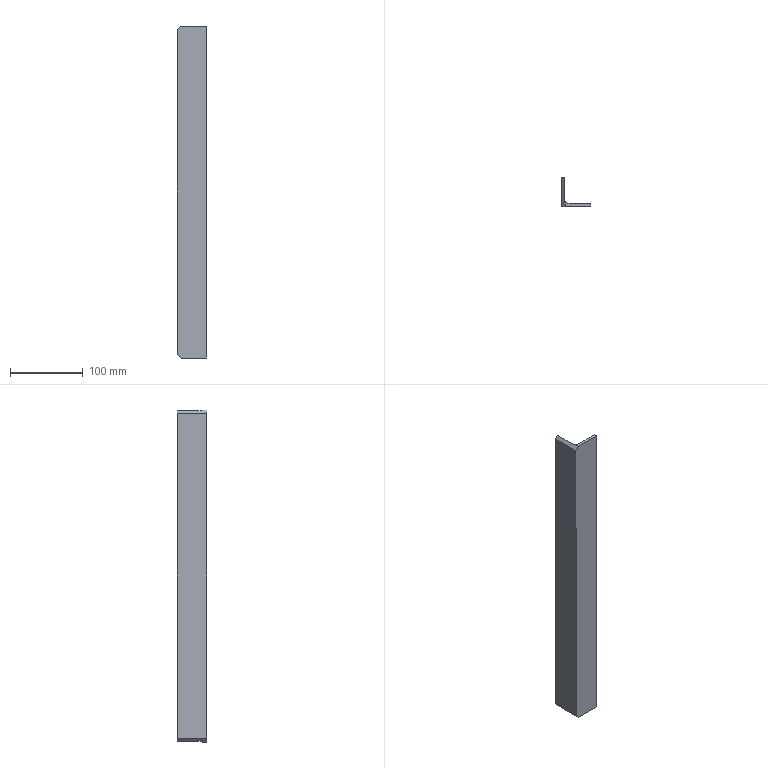Part | SolidWorks | features Cut 1, Extrusion 1 | 1 solid | 13 faces | box 40 x 40 x 456 mm | volume 140103 mm3 | plane 10 | cylinder 3 | commonest cylinder face diameters 0.02 x2 10 x1
STEP:
#1=CARTESIAN_POINT('',(0.,0.,451.));
#2=VERTEX_POINT('',#1);
#3=CARTESIAN_POINT('',(0.,0.,5.));
#4=VERTEX_POINT('',#3);
#5=CARTESIAN_POINT('',(0.,0.,456.));
#6=DIRECTION('',(0.,0.,-1.));
#7=VECTOR('',#6,1000.);
#8=LINE('',#5,#7);
#9=EDGE_CURVE('',#2,#4,#8,.T.);
#10=ORIENTED_EDGE('',*,*,#9,.T.);
#11=CARTESIAN_POINT('',(5.,0.,0.));
#12=VERTEX_POINT('',#11);
#13=CARTESIAN_POINT('',(0.,0.,5.));
#14=DIRECTION('',(0.7071,0.,-0.7071));
#15=VECTOR('',#14,1000.);
#16=LINE('',#13,#15);
#17=EDGE_CURVE('',#4,#12,#16,.T.);
#18=ORIENTED_EDGE('',*,*,#17,.T.);
#19=CARTESIAN_POINT('',(40.,0.,0.));
#20=VERTEX_POINT('',#19);
#21=CARTESIAN_POINT('',(40.,0.,0.));
#22=DIRECTION('',(1.,0.,0.));
#23=VECTOR('',#22,1000.);
#24=LINE('',#21,#23);
#25=EDGE_CURVE('',#12,#20,#24,.T.);
#26=ORIENTED_EDGE('',*,*,#25,.T.);
#27=CARTESIAN_POINT('',(40.,0.,456.));
#28=VERTEX_POINT('',#27);
#29=CARTESIAN_POINT('',(40.,0.,456.));
#30=DIRECTION('',(0.,0.,-1.));
#31=VECTOR('',#30,1000.);
#32=LINE('',#29,#31);
#33=EDGE_CURVE('',#28,#20,#32,.T.);
#34=ORIENTED_EDGE('',*,*,#33,.F.);
#35=CARTESIAN_POINT('',(5.,0.,456.));
#36=VERTEX_POINT('',#35);
#37=CARTESIAN_POINT('',(40.,0.,456.));
#38=DIRECTION('',(1.,0.,0.));
#39=VECTOR('',#38,1000.);
#40=LINE('',#37,#39);
#41=EDGE_CURVE('',#36,#28,#40,.T.);
#42=ORIENTED_EDGE('',*,*,#41,.F.);
#43=CARTESIAN_POINT('',(5.,0.,456.));
#44=DIRECTION('',(-0.7071,0.,-0.7071));
#45=VECTOR('',#44,1000.);
#46=LINE('',#43,#45);
#47=EDGE_CURVE('',#36,#2,#46,.T.);
#48=ORIENTED_EDGE('',*,*,#47,.T.);
#49=EDGE_LOOP('',(#10,#18,#26,#34,#42,#48));
#50=FACE_OUTER_BOUND('',#49,.T.);
#51=CARTESIAN_POINT('',(40.,0.,456.));
#52=DIRECTION('',(0.,1.,0.));
#53=DIRECTION('',(-1.,0.,0.));
#54=AXIS2_PLACEMENT_3D('',#51,#52,#53);
#55=PLANE('',#54);
#56=ADVANCED_FACE('',(#50),#55,.F.);
#57=CARTESIAN_POINT('',(40.,3.99,0.));
#58=VERTEX_POINT('',#57);
#59=CARTESIAN_POINT('',(40.,3.99,0.));
#60=DIRECTION('',(0.,1.,0.));
#61=VECTOR('',#60,1000.);
#62=LINE('',#59,#61);
#63=EDGE_CURVE('',#20,#58,#62,.T.);
#64=ORIENTED_EDGE('',*,*,#63,.T.);
#65=CARTESIAN_POINT('',(40.,3.99,456.));
#66=VERTEX_POINT('',#65);
#67=CARTESIAN_POINT('',(40.,3.99,456.));
#68=DIRECTION('',(0.,0.,-1.));
#69=VECTOR('',#68,1000.);
#70=LINE('',#67,#69);
#71=EDGE_CURVE('',#66,#58,#70,.T.);
#72=ORIENTED_EDGE('',*,*,#71,.F.);
#73=CARTESIAN_POINT('',(40.,3.99,456.));
#74=DIRECTION('',(0.,1.,0.));
#75=VECTOR('',#74,1000.);
#76=LINE('',#73,#75);
#77=EDGE_CURVE('',#28,#66,#76,.T.);
#78=ORIENTED_EDGE('',*,*,#77,.F.);
#79=ORIENTED_EDGE('',*,*,#33,.T.);
#80=EDGE_LOOP('',(#64,#72,#78,#79));
#81=FACE_OUTER_BOUND('',#80,.T.);
#82=CARTESIAN_POINT('',(40.,3.99,456.));
#83=DIRECTION('',(-1.,0.,0.));
#84=DIRECTION('',(0.,0.,1.));
#85=AXIS2_PLACEMENT_3D('',#82,#83,#84);
#86=PLANE('',#85);
#87=ADVANCED_FACE('',(#81),#86,.F.);
#88=CARTESIAN_POINT('',(39.99,4.,0.));
#89=VERTEX_POINT('',#88);
#90=CARTESIAN_POINT('',(39.99,3.99,0.));
#91=DIRECTION('',(0.,0.,1.));
#92=DIRECTION('',(1.,0.,0.));
#93=AXIS2_PLACEMENT_3D('',#90,#91,#92);
#94=CIRCLE('',#93,0.01);
#95=EDGE_CURVE('',#58,#89,#94,.T.);
#96=ORIENTED_EDGE('',*,*,#95,.T.);
#97=CARTESIAN_POINT('',(39.99,4.,456.));
#98=VERTEX_POINT('',#97);
#99=CARTESIAN_POINT('',(39.99,4.,456.));
#100=DIRECTION('',(0.,0.,-1.));
#101=VECTOR('',#100,1000.);
#102=LINE('',#99,#101);
#103=EDGE_CURVE('',#98,#89,#102,.T.);
#104=ORIENTED_EDGE('',*,*,#103,.F.);
#105=CARTESIAN_POINT('',(39.99,3.99,456.));
#106=DIRECTION('',(0.,0.,1.));
#107=DIRECTION('',(1.,0.,0.));
#108=AXIS2_PLACEMENT_3D('',#105,#106,#107);
#109=CIRCLE('',#108,0.01);
#110=EDGE_CURVE('',#66,#98,#109,.T.);
#111=ORIENTED_EDGE('',*,*,#110,.F.);
#112=ORIENTED_EDGE('',*,*,#71,.T.);
#113=EDGE_LOOP('',(#96,#104,#111,#112));
#114=FACE_OUTER_BOUND('',#113,.T.);
#115=CARTESIAN_POINT('',(39.99,3.99,456.));
#116=DIRECTION('',(0.,0.,-1.));
#117=DIRECTION('',(-1.,0.,0.));
#118=AXIS2_PLACEMENT_3D('',#115,#116,#117);
#119=CYLINDRICAL_SURFACE('',#118,0.01);
#120=ADVANCED_FACE('',(#114),#119,.T.);
#121=CARTESIAN_POINT('',(9.,4.,0.));
#122=VERTEX_POINT('',#121);
#123=CARTESIAN_POINT('',(9.,4.,0.));
#124=DIRECTION('',(-1.,0.,0.));
#125=VECTOR('',#124,1000.);
#126=LINE('',#123,#125);
#127=EDGE_CURVE('',#89,#122,#126,.T.);
#128=ORIENTED_EDGE('',*,*,#127,.T.);
#129=CARTESIAN_POINT('',(9.,4.,456.));
#130=VERTEX_POINT('',#129);
#131=CARTESIAN_POINT('',(9.,4.,456.));
#132=DIRECTION('',(0.,0.,-1.));
#133=VECTOR('',#132,1000.);
#134=LINE('',#131,#133);
#135=EDGE_CURVE('',#130,#122,#134,.T.);
#136=ORIENTED_EDGE('',*,*,#135,.F.);
#137=CARTESIAN_POINT('',(9.,4.,456.));
#138=DIRECTION('',(-1.,0.,0.));
#139=VECTOR('',#138,1000.);
#140=LINE('',#137,#139);
#141=EDGE_CURVE('',#98,#130,#140,.T.);
#142=ORIENTED_EDGE('',*,*,#141,.F.);
#143=ORIENTED_EDGE('',*,*,#103,.T.);
#144=EDGE_LOOP('',(#128,#136,#142,#143));
#145=FACE_OUTER_BOUND('',#144,.T.);
#146=CARTESIAN_POINT('',(9.,4.,456.));
#147=DIRECTION('',(0.,-1.,0.));
#148=DIRECTION('',(0.,0.,-1.));
#149=AXIS2_PLACEMENT_3D('',#146,#147,#148);
#150=PLANE('',#149);
#151=ADVANCED_FACE('',(#145),#150,.F.);
#152=CARTESIAN_POINT('',(5.,6.,0.));
#153=VERTEX_POINT('',#152);
#154=CARTESIAN_POINT('',(9.,9.,0.));
#155=DIRECTION('',(0.,0.,-1.));
#156=DIRECTION('',(-1.,0.,0.));
#157=AXIS2_PLACEMENT_3D('',#154,#155,#156);
#158=CIRCLE('',#157,5.);
#159=EDGE_CURVE('',#122,#153,#158,.T.);
#160=ORIENTED_EDGE('',*,*,#159,.T.);
#161=CARTESIAN_POINT('',(4.,9.,1.));
#162=VERTEX_POINT('',#161);
#163=CARTESIAN_POINT('',(5.,6.,0.));
#164=CARTESIAN_POINT('',(4.345,6.873,0.6549));
#165=CARTESIAN_POINT('',(4.,7.909,1.));
#166=CARTESIAN_POINT('',(4.,9.,1.));
#167=(BOUNDED_CURVE()B_SPLINE_CURVE(3,(#163,#164,#165,#166),.UNSPECIFIED.,.F.,.F.)B_SPLINE_CURVE_WITH_KNOTS((4,4),(2.498,3.142),.UNSPECIFIED.)CURVE()GEOMETRIC_REPRESENTATION_ITEM()RATIONAL_B_SPLINE_CURVE((1.,0.9658,0.9658,1.))REPRESENTATION_ITEM(''));
#168=EDGE_CURVE('',#153,#162,#167,.T.);
#169=ORIENTED_EDGE('',*,*,#168,.T.);
#170=CARTESIAN_POINT('',(4.,9.,455.));
#171=VERTEX_POINT('',#170);
#172=CARTESIAN_POINT('',(4.,9.,456.));
#173=DIRECTION('',(0.,0.,-1.));
#174=VECTOR('',#173,1000.);
#175=LINE('',#172,#174);
#176=EDGE_CURVE('',#171,#162,#175,.T.);
#177=ORIENTED_EDGE('',*,*,#176,.F.);
#178=CARTESIAN_POINT('',(5.,6.,456.));
#179=VERTEX_POINT('',#178);
#180=CARTESIAN_POINT('',(4.,9.,455.));
#181=CARTESIAN_POINT('',(4.,7.909,455.));
#182=CARTESIAN_POINT('',(4.345,6.873,455.345));
#183=CARTESIAN_POINT('',(5.,6.,456.));
#184=(BOUNDED_CURVE()B_SPLINE_CURVE(3,(#180,#181,#182,#183),.UNSPECIFIED.,.F.,.T.)B_SPLINE_CURVE_WITH_KNOTS((4,4),(0.,0.6435),.UNSPECIFIED.)CURVE()GEOMETRIC_REPRESENTATION_ITEM()RATIONAL_B_SPLINE_CURVE((1.,0.9658,0.9658,1.))REPRESENTATION_ITEM(''));
#185=EDGE_CURVE('',#171,#179,#184,.T.);
#186=ORIENTED_EDGE('',*,*,#185,.T.);
#187=CARTESIAN_POINT('',(9.,9.,456.));
#188=DIRECTION('',(0.,0.,-1.));
#189=DIRECTION('',(-1.,0.,0.));
#190=AXIS2_PLACEMENT_3D('',#187,#188,#189);
#191=CIRCLE('',#190,5.);
#192=EDGE_CURVE('',#130,#179,#191,.T.);
#193=ORIENTED_EDGE('',*,*,#192,.F.);
#194=ORIENTED_EDGE('',*,*,#135,.T.);
#195=EDGE_LOOP('',(#160,#169,#177,#186,#193,#194));
#196=FACE_OUTER_BOUND('',#195,.T.);
#197=CARTESIAN_POINT('',(9.,9.,456.));
#198=DIRECTION('',(0.,0.,-1.));
#199=DIRECTION('',(-1.,0.,0.));
#200=AXIS2_PLACEMENT_3D('',#197,#198,#199);
#201=CYLINDRICAL_SURFACE('',#200,5.);
#202=ADVANCED_FACE('',(#196),#201,.F.);
#203=ORIENTED_EDGE('',*,*,#176,.T.);
#204=CARTESIAN_POINT('',(4.,39.99,1.));
#205=VERTEX_POINT('',#204);
#206=CARTESIAN_POINT('',(4.,39.99,1.));
#207=DIRECTION('',(0.,1.,0.));
#208=VECTOR('',#207,1000.);
#209=LINE('',#206,#208);
#210=EDGE_CURVE('',#162,#205,#209,.T.);
#211=ORIENTED_EDGE('',*,*,#210,.T.);
#212=CARTESIAN_POINT('',(4.,39.99,455.));
#213=VERTEX_POINT('',#212);
#214=CARTESIAN_POINT('',(4.,39.99,456.));
#215=DIRECTION('',(0.,0.,-1.));
#216=VECTOR('',#215,1000.);
#217=LINE('',#214,#216);
#218=EDGE_CURVE('',#213,#205,#217,.T.);
#219=ORIENTED_EDGE('',*,*,#218,.F.);
#220=CARTESIAN_POINT('',(4.,39.99,455.));
#221=DIRECTION('',(0.,-1.,0.));
#222=VECTOR('',#221,1000.);
#223=LINE('',#220,#222);
#224=EDGE_CURVE('',#213,#171,#223,.T.);
#225=ORIENTED_EDGE('',*,*,#224,.T.);
#226=EDGE_LOOP('',(#203,#211,#219,#225));
#227=FACE_OUTER_BOUND('',#226,.T.);
#228=CARTESIAN_POINT('',(4.,39.99,456.));
#229=DIRECTION('',(-1.,0.,0.));
#230=DIRECTION('',(0.,-1.,0.));
#231=AXIS2_PLACEMENT_3D('',#228,#229,#230);
#232=PLANE('',#231);
#233=ADVANCED_FACE('',(#227),#232,.F.);
#234=ORIENTED_EDGE('',*,*,#218,.T.);
#235=CARTESIAN_POINT('',(3.99,40.,1.01));
#236=VERTEX_POINT('',#235);
#237=CARTESIAN_POINT('',(4.,39.99,1.));
#238=CARTESIAN_POINT('',(4.,39.996,1.));
#239=CARTESIAN_POINT('',(3.996,40.,1.004));
#240=CARTESIAN_POINT('',(3.99,40.,1.01));
#241=(BOUNDED_CURVE()B_SPLINE_CURVE(3,(#237,#238,#239,#240),.UNSPECIFIED.,.F.,.T.)B_SPLINE_CURVE_WITH_KNOTS((4,4),(0.,1.571),.UNSPECIFIED.)CURVE()GEOMETRIC_REPRESENTATION_ITEM()RATIONAL_B_SPLINE_CURVE((1.,0.8047,0.8047,1.))REPRESENTATION_ITEM(''));
#242=EDGE_CURVE('',#205,#236,#241,.T.);
#243=ORIENTED_EDGE('',*,*,#242,.T.);
#244=CARTESIAN_POINT('',(3.99,40.,454.99));
#245=VERTEX_POINT('',#244);
#246=CARTESIAN_POINT('',(3.99,40.,456.));
#247=DIRECTION('',(0.,0.,-1.));
#248=VECTOR('',#247,1000.);
#249=LINE('',#246,#248);
#250=EDGE_CURVE('',#245,#236,#249,.T.);
#251=ORIENTED_EDGE('',*,*,#250,.F.);
#252=CARTESIAN_POINT('',(3.99,40.,454.99));
#253=CARTESIAN_POINT('',(3.996,40.,454.996));
#254=CARTESIAN_POINT('',(4.,39.996,455.));
#255=CARTESIAN_POINT('',(4.,39.99,455.));
#256=(BOUNDED_CURVE()B_SPLINE_CURVE(3,(#252,#253,#254,#255),.UNSPECIFIED.,.F.,.F.)B_SPLINE_CURVE_WITH_KNOTS((4,4),(1.571,3.142),.UNSPECIFIED.)CURVE()GEOMETRIC_REPRESENTATION_ITEM()RATIONAL_B_SPLINE_CURVE((1.,0.8047,0.8047,1.))REPRESENTATION_ITEM(''));
#257=EDGE_CURVE('',#245,#213,#256,.T.);
#258=ORIENTED_EDGE('',*,*,#257,.T.);
#259=EDGE_LOOP('',(#234,#243,#251,#258));
#260=FACE_OUTER_BOUND('',#259,.T.);
#261=CARTESIAN_POINT('',(3.99,39.99,456.));
#262=DIRECTION('',(0.,0.,-1.));
#263=DIRECTION('',(-1.,0.,0.));
#264=AXIS2_PLACEMENT_3D('',#261,#262,#263);
#265=CYLINDRICAL_SURFACE('',#264,0.01);
#266=ADVANCED_FACE('',(#260),#265,.T.);
#267=ORIENTED_EDGE('',*,*,#250,.T.);
#268=CARTESIAN_POINT('',(0.,40.,5.));
#269=VERTEX_POINT('',#268);
#270=CARTESIAN_POINT('',(0.,40.,5.));
#271=DIRECTION('',(0.7071,0.,-0.7071));
#272=VECTOR('',#271,1000.);
#273=LINE('',#270,#272);
#274=EDGE_CURVE('',#269,#236,#273,.T.);
#275=ORIENTED_EDGE('',*,*,#274,.F.);
#276=CARTESIAN_POINT('',(0.,40.,451.));
#277=VERTEX_POINT('',#276);
#278=CARTESIAN_POINT('',(0.,40.,456.));
#279=DIRECTION('',(0.,0.,-1.));
#280=VECTOR('',#279,1000.);
#281=LINE('',#278,#280);
#282=EDGE_CURVE('',#277,#269,#281,.T.);
#283=ORIENTED_EDGE('',*,*,#282,.F.);
#284=CARTESIAN_POINT('',(5.,40.,456.));
#285=DIRECTION('',(-0.7071,0.,-0.7071));
#286=VECTOR('',#285,1000.);
#287=LINE('',#284,#286);
#288=EDGE_CURVE('',#245,#277,#287,.T.);
#289=ORIENTED_EDGE('',*,*,#288,.F.);
#290=EDGE_LOOP('',(#267,#275,#283,#289));
#291=FACE_OUTER_BOUND('',#290,.T.);
#292=CARTESIAN_POINT('',(0.,40.,456.));
#293=DIRECTION('',(0.,-1.,0.));
#294=DIRECTION('',(0.,0.,-1.));
#295=AXIS2_PLACEMENT_3D('',#292,#293,#294);
#296=PLANE('',#295);
#297=ADVANCED_FACE('',(#291),#296,.F.);
#298=ORIENTED_EDGE('',*,*,#282,.T.);
#299=CARTESIAN_POINT('',(0.,0.,5.));
#300=DIRECTION('',(0.,1.,0.));
#301=VECTOR('',#300,1000.);
#302=LINE('',#299,#301);
#303=EDGE_CURVE('',#4,#269,#302,.T.);
#304=ORIENTED_EDGE('',*,*,#303,.F.);
#305=ORIENTED_EDGE('',*,*,#9,.F.);
#306=CARTESIAN_POINT('',(0.,0.,451.));
#307=DIRECTION('',(0.,1.,0.));
#308=VECTOR('',#307,1000.);
#309=LINE('',#306,#308);
#310=EDGE_CURVE('',#2,#277,#309,.T.);
#311=ORIENTED_EDGE('',*,*,#310,.T.);
#312=EDGE_LOOP('',(#298,#304,#305,#311));
#313=FACE_OUTER_BOUND('',#312,.T.);
#314=CARTESIAN_POINT('',(0.,0.,456.));
#315=DIRECTION('',(1.,0.,0.));
#316=DIRECTION('',(0.,0.,-1.));
#317=AXIS2_PLACEMENT_3D('',#314,#315,#316);
#318=PLANE('',#317);
#319=ADVANCED_FACE('',(#313),#318,.F.);
#320=CARTESIAN_POINT('',(5.,0.,456.));
#321=DIRECTION('',(0.,1.,0.));
#322=VECTOR('',#321,1000.);
#323=LINE('',#320,#322);
#324=EDGE_CURVE('',#36,#179,#323,.T.);
#325=ORIENTED_EDGE('',*,*,#324,.F.);
#326=ORIENTED_EDGE('',*,*,#41,.T.);
#327=ORIENTED_EDGE('',*,*,#77,.T.);
#328=ORIENTED_EDGE('',*,*,#110,.T.);
#329=ORIENTED_EDGE('',*,*,#141,.T.);
#330=ORIENTED_EDGE('',*,*,#192,.T.);
#331=EDGE_LOOP('',(#325,#326,#327,#328,#329,#330));
#332=FACE_OUTER_BOUND('',#331,.T.);
#333=CARTESIAN_POINT('',(3.99,39.99,456.));
#334=DIRECTION('',(0.,0.,1.));
#335=DIRECTION('',(1.,0.,0.));
#336=AXIS2_PLACEMENT_3D('',#333,#334,#335);
#337=PLANE('',#336);
#338=ADVANCED_FACE('',(#332),#337,.T.);
#339=ORIENTED_EDGE('',*,*,#25,.F.);
#340=CARTESIAN_POINT('',(5.,0.,0.));
#341=DIRECTION('',(0.,1.,0.));
#342=VECTOR('',#341,1000.);
#343=LINE('',#340,#342);
#344=EDGE_CURVE('',#12,#153,#343,.T.);
#345=ORIENTED_EDGE('',*,*,#344,.T.);
#346=ORIENTED_EDGE('',*,*,#159,.F.);
#347=ORIENTED_EDGE('',*,*,#127,.F.);
#348=ORIENTED_EDGE('',*,*,#95,.F.);
#349=ORIENTED_EDGE('',*,*,#63,.F.);
#350=EDGE_LOOP('',(#339,#345,#346,#347,#348,#349));
#351=FACE_OUTER_BOUND('',#350,.T.);
#352=CARTESIAN_POINT('',(3.99,39.99,0.));
#353=DIRECTION('',(0.,0.,1.));
#354=DIRECTION('',(1.,0.,0.));
#355=AXIS2_PLACEMENT_3D('',#352,#353,#354);
#356=PLANE('',#355);
#357=ADVANCED_FACE('',(#351),#356,.F.);
#358=ORIENTED_EDGE('',*,*,#224,.F.);
#359=ORIENTED_EDGE('',*,*,#257,.F.);
#360=ORIENTED_EDGE('',*,*,#288,.T.);
#361=ORIENTED_EDGE('',*,*,#310,.F.);
#362=ORIENTED_EDGE('',*,*,#47,.F.);
#363=ORIENTED_EDGE('',*,*,#324,.T.);
#364=ORIENTED_EDGE('',*,*,#185,.F.);
#365=EDGE_LOOP('',(#358,#359,#360,#361,#362,#363,#364));
#366=FACE_OUTER_BOUND('',#365,.T.);
#367=CARTESIAN_POINT('',(5.,0.,456.));
#368=DIRECTION('',(0.7071,0.,-0.7071));
#369=DIRECTION('',(-0.7071,0.,-0.7071));
#370=AXIS2_PLACEMENT_3D('',#367,#368,#369);
#371=PLANE('',#370);
#372=ADVANCED_FACE('',(#366),#371,.F.);
#373=ORIENTED_EDGE('',*,*,#344,.F.);
#374=ORIENTED_EDGE('',*,*,#17,.F.);
#375=ORIENTED_EDGE('',*,*,#303,.T.);
#376=ORIENTED_EDGE('',*,*,#274,.T.);
#377=ORIENTED_EDGE('',*,*,#242,.F.);
#378=ORIENTED_EDGE('',*,*,#210,.F.);
#379=ORIENTED_EDGE('',*,*,#168,.F.);
#380=EDGE_LOOP('',(#373,#374,#375,#376,#377,#378,#379));
#381=FACE_OUTER_BOUND('',#380,.T.);
#382=CARTESIAN_POINT('',(0.,0.,5.));
#383=DIRECTION('',(0.7071,0.,0.7071));
#384=DIRECTION('',(0.7071,0.,-0.7071));
#385=AXIS2_PLACEMENT_3D('',#382,#383,#384);
#386=PLANE('',#385);
#387=ADVANCED_FACE('',(#381),#386,.F.);
#388=CLOSED_SHELL('',(#56,#87,#120,#151,#202,#233,#266,#297,#319,#338,#357,#372,#387));
#389=MANIFOLD_SOLID_BREP('',#388);
#390=CARTESIAN_POINT('',(0.,0.,0.));
#391=DIRECTION('',(0.,0.,1.));
#392=DIRECTION('',(1.,0.,0.));
#393=AXIS2_PLACEMENT_3D('',#390,#391,#392);
#394=(LENGTH_UNIT()NAMED_UNIT(*)SI_UNIT(.MILLI.,.METRE.));
#395=UNCERTAINTY_MEASURE_WITH_UNIT(LENGTH_MEASURE(0.00001),#394,'','');
#396=(NAMED_UNIT(*)PLANE_ANGLE_UNIT()SI_UNIT($,.RADIAN.));
#397=(NAMED_UNIT(*)SI_UNIT($,.STERADIAN.)SOLID_ANGLE_UNIT());
#398=(GEOMETRIC_REPRESENTATION_CONTEXT(3)GLOBAL_UNCERTAINTY_ASSIGNED_CONTEXT((#395))GLOBAL_UNIT_ASSIGNED_CONTEXT((#394,#396,#397))REPRESENTATION_CONTEXT('',''));
#399=ADVANCED_BREP_SHAPE_REPRESENTATION('',(#389,#393),#398);